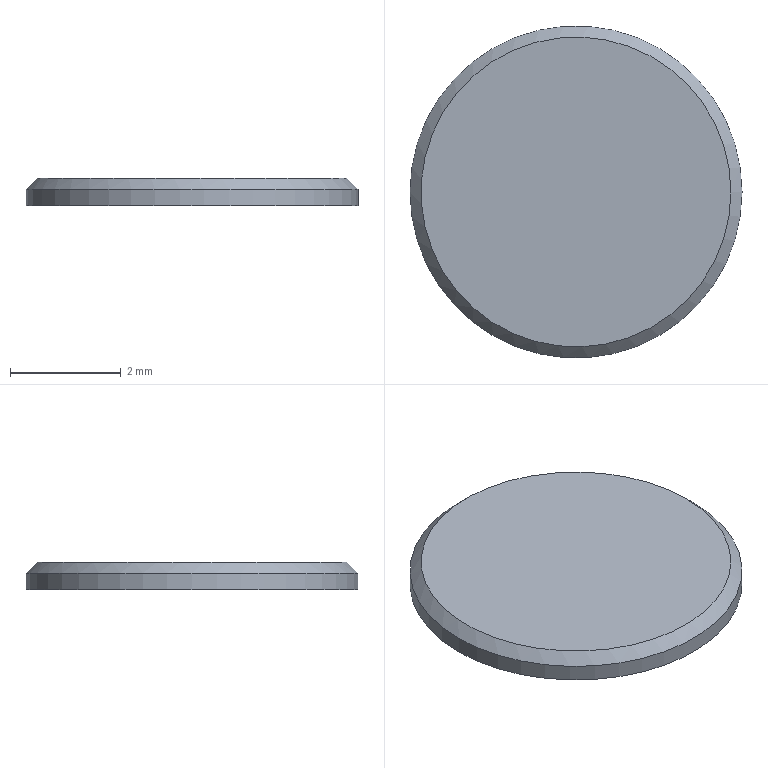Part | NX | features DATUM_CSYS 2, CHAMFER 1, EXTRUDE 1, SKETCH 1 | 1 solid | 4 faces | box 6 x 6 x 0.5 mm | volume 13.769 mm3 | plane 2 | cylinder 1 | cone 1 | commonest cylinder face diameters 6 x1
STEP:
#1=CARTESIAN_POINT('',(3.,0.,0.3));
#2=VERTEX_POINT('',#1);
#3=CARTESIAN_POINT('',(0.,0.,0.3));
#4=DIRECTION('',(0.,0.,1.));
#5=DIRECTION('',(1.,0.,0.));
#6=AXIS2_PLACEMENT_3D('',#3,#4,#5);
#7=CIRCLE('',#6,3.);
#8=EDGE_CURVE('',#2,#2,#7,.F.);
#9=ORIENTED_EDGE('',*,*,#8,.T.);
#10=EDGE_LOOP('',(#9));
#11=FACE_BOUND('',#10,.T.);
#12=CARTESIAN_POINT('',(3.,0.,0.));
#13=VERTEX_POINT('',#12);
#14=CARTESIAN_POINT('',(0.,0.,0.));
#15=DIRECTION('',(0.,0.,1.));
#16=DIRECTION('',(1.,0.,0.));
#17=AXIS2_PLACEMENT_3D('',#14,#15,#16);
#18=CIRCLE('',#17,3.);
#19=EDGE_CURVE('',#13,#13,#18,.T.);
#20=ORIENTED_EDGE('',*,*,#19,.T.);
#21=EDGE_LOOP('',(#20));
#22=FACE_BOUND('',#21,.T.);
#23=CARTESIAN_POINT('',(0.,0.,0.5));
#24=DIRECTION('',(0.,0.,-1.));
#25=DIRECTION('',(-1.,0.,0.));
#26=AXIS2_PLACEMENT_3D('',#23,#24,#25);
#27=CYLINDRICAL_SURFACE('',#26,3.);
#28=ADVANCED_FACE('',(#11,#22),#27,.T.);
#29=CARTESIAN_POINT('',(2.8,0.,0.5));
#30=VERTEX_POINT('',#29);
#31=CARTESIAN_POINT('',(0.,0.,0.5));
#32=DIRECTION('',(0.,0.,1.));
#33=DIRECTION('',(1.,0.,0.));
#34=AXIS2_PLACEMENT_3D('',#31,#32,#33);
#35=CIRCLE('',#34,2.8);
#36=EDGE_CURVE('',#30,#30,#35,.T.);
#37=ORIENTED_EDGE('',*,*,#36,.T.);
#38=EDGE_LOOP('',(#37));
#39=FACE_BOUND('',#38,.T.);
#40=CARTESIAN_POINT('',(0.,0.,0.5));
#41=DIRECTION('',(0.,0.,1.));
#42=DIRECTION('',(1.,0.,0.));
#43=AXIS2_PLACEMENT_3D('',#40,#41,#42);
#44=PLANE('',#43);
#45=ADVANCED_FACE('',(#39),#44,.T.);
#46=ORIENTED_EDGE('',*,*,#19,.F.);
#47=EDGE_LOOP('',(#46));
#48=FACE_BOUND('',#47,.T.);
#49=CARTESIAN_POINT('',(0.,0.,0.));
#50=DIRECTION('',(0.,0.,1.));
#51=DIRECTION('',(1.,0.,0.));
#52=AXIS2_PLACEMENT_3D('',#49,#50,#51);
#53=PLANE('',#52);
#54=ADVANCED_FACE('',(#48),#53,.F.);
#55=ORIENTED_EDGE('',*,*,#8,.F.);
#56=EDGE_LOOP('',(#55));
#57=FACE_BOUND('',#56,.T.);
#58=ORIENTED_EDGE('',*,*,#36,.F.);
#59=EDGE_LOOP('',(#58));
#60=FACE_BOUND('',#59,.T.);
#61=CARTESIAN_POINT('',(0.,0.,0.5));
#62=DIRECTION('',(0.,0.,-1.));
#63=DIRECTION('',(-1.,0.,0.));
#64=AXIS2_PLACEMENT_3D('',#61,#62,#63);
#65=CONICAL_SURFACE('',#64,2.8,0.7854);
#66=ADVANCED_FACE('',(#57,#60),#65,.T.);
#67=CLOSED_SHELL('',(#28,#45,#54,#66));
#68=MANIFOLD_SOLID_BREP('',#67);
#69=(LENGTH_UNIT()NAMED_UNIT(*)SI_UNIT(.MILLI.,.METRE.));
#70=UNCERTAINTY_MEASURE_WITH_UNIT(LENGTH_MEASURE(0.00001),#69,'','');
#71=(NAMED_UNIT(*)PLANE_ANGLE_UNIT()SI_UNIT($,.RADIAN.));
#72=(NAMED_UNIT(*)SI_UNIT($,.STERADIAN.)SOLID_ANGLE_UNIT());
#73=(GEOMETRIC_REPRESENTATION_CONTEXT(3)GLOBAL_UNCERTAINTY_ASSIGNED_CONTEXT((#70))GLOBAL_UNIT_ASSIGNED_CONTEXT((#69,#71,#72))REPRESENTATION_CONTEXT('',''));
#74=ADVANCED_BREP_SHAPE_REPRESENTATION('',(#68),#73);